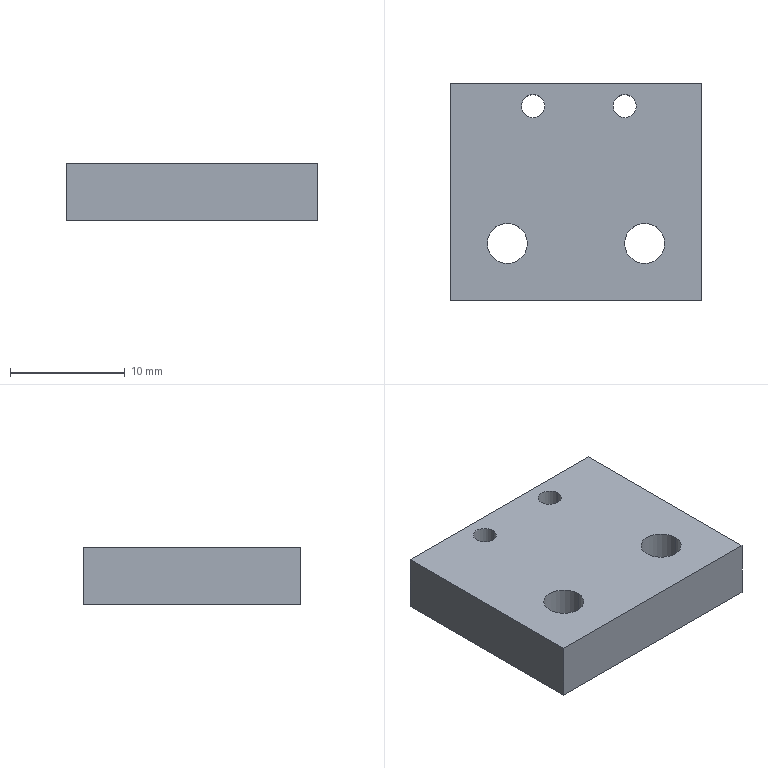Part | SolidWorks | features BaseBody 1 | 1 solid | 14 faces | box 22 x 19 x 5 mm | volume 1962 mm3 | cylinder 8 | plane 6 | commonest cylinder face diameters 2.013 x4 3.5 x4
STEP:
#1=CARTESIAN_POINT('',(-23.757,7.,0.));
#2=VERTEX_POINT('',#1);
#3=CARTESIAN_POINT('',(-21.744,7.,0.));
#4=VERTEX_POINT('',#3);
#5=CARTESIAN_POINT('',(-22.75,7.,0.));
#6=DIRECTION('',(0.,0.,1.));
#7=DIRECTION('',(1.,0.,0.));
#8=AXIS2_PLACEMENT_3D('',#5,#6,#7);
#9=CIRCLE('',#8,1.007);
#10=EDGE_CURVE('',#2,#4,#9,.T.);
#11=ORIENTED_EDGE('',*,*,#10,.F.);
#12=CARTESIAN_POINT('',(-23.757,7.,5.));
#13=VERTEX_POINT('',#12);
#14=CARTESIAN_POINT('',(-23.757,7.,-24.496));
#15=DIRECTION('',(0.,0.,1.));
#16=VECTOR('',#15,1000.);
#17=LINE('',#14,#16);
#18=EDGE_CURVE('',#2,#13,#17,.T.);
#19=ORIENTED_EDGE('',*,*,#18,.T.);
#20=CARTESIAN_POINT('',(-21.744,7.,5.));
#21=VERTEX_POINT('',#20);
#22=CARTESIAN_POINT('',(-22.75,7.,5.));
#23=DIRECTION('',(0.,0.,-1.));
#24=DIRECTION('',(1.,0.,0.));
#25=AXIS2_PLACEMENT_3D('',#22,#23,#24);
#26=CIRCLE('',#25,1.007);
#27=EDGE_CURVE('',#21,#13,#26,.T.);
#28=ORIENTED_EDGE('',*,*,#27,.F.);
#29=CARTESIAN_POINT('',(-21.744,7.,-24.496));
#30=DIRECTION('',(0.,0.,1.));
#31=VECTOR('',#30,1000.);
#32=LINE('',#29,#31);
#33=EDGE_CURVE('',#4,#21,#32,.T.);
#34=ORIENTED_EDGE('',*,*,#33,.F.);
#35=EDGE_LOOP('',(#11,#19,#28,#34));
#36=FACE_OUTER_BOUND('',#35,.T.);
#37=CARTESIAN_POINT('',(-22.75,7.,-24.496));
#38=DIRECTION('',(0.,0.,1.));
#39=DIRECTION('',(1.,0.,0.));
#40=AXIS2_PLACEMENT_3D('',#37,#38,#39);
#41=CYLINDRICAL_SURFACE('',#40,1.007);
#42=ADVANCED_FACE('',(#36),#41,.F.);
#43=CARTESIAN_POINT('',(-15.757,7.,0.));
#44=VERTEX_POINT('',#43);
#45=CARTESIAN_POINT('',(-13.744,7.,0.));
#46=VERTEX_POINT('',#45);
#47=CARTESIAN_POINT('',(-14.75,7.,0.));
#48=DIRECTION('',(0.,0.,1.));
#49=DIRECTION('',(1.,0.,0.));
#50=AXIS2_PLACEMENT_3D('',#47,#48,#49);
#51=CIRCLE('',#50,1.007);
#52=EDGE_CURVE('',#44,#46,#51,.T.);
#53=ORIENTED_EDGE('',*,*,#52,.F.);
#54=CARTESIAN_POINT('',(-15.757,7.,5.));
#55=VERTEX_POINT('',#54);
#56=CARTESIAN_POINT('',(-15.757,7.,-24.496));
#57=DIRECTION('',(0.,0.,1.));
#58=VECTOR('',#57,1000.);
#59=LINE('',#56,#58);
#60=EDGE_CURVE('',#44,#55,#59,.T.);
#61=ORIENTED_EDGE('',*,*,#60,.T.);
#62=CARTESIAN_POINT('',(-13.744,7.,5.));
#63=VERTEX_POINT('',#62);
#64=CARTESIAN_POINT('',(-14.75,7.,5.));
#65=DIRECTION('',(0.,0.,-1.));
#66=DIRECTION('',(1.,0.,0.));
#67=AXIS2_PLACEMENT_3D('',#64,#65,#66);
#68=CIRCLE('',#67,1.007);
#69=EDGE_CURVE('',#63,#55,#68,.T.);
#70=ORIENTED_EDGE('',*,*,#69,.F.);
#71=CARTESIAN_POINT('',(-13.744,7.,-24.496));
#72=DIRECTION('',(0.,0.,1.));
#73=VECTOR('',#72,1000.);
#74=LINE('',#71,#73);
#75=EDGE_CURVE('',#46,#63,#74,.T.);
#76=ORIENTED_EDGE('',*,*,#75,.F.);
#77=EDGE_LOOP('',(#53,#61,#70,#76));
#78=FACE_OUTER_BOUND('',#77,.T.);
#79=CARTESIAN_POINT('',(-14.75,7.,-24.496));
#80=DIRECTION('',(0.,0.,1.));
#81=DIRECTION('',(1.,0.,0.));
#82=AXIS2_PLACEMENT_3D('',#79,#80,#81);
#83=CYLINDRICAL_SURFACE('',#82,1.007);
#84=ADVANCED_FACE('',(#78),#83,.F.);
#85=CARTESIAN_POINT('',(-26.75,-5.,0.));
#86=VERTEX_POINT('',#85);
#87=CARTESIAN_POINT('',(-23.25,-5.,0.));
#88=VERTEX_POINT('',#87);
#89=CARTESIAN_POINT('',(-25.,-5.,0.));
#90=DIRECTION('',(0.,0.,1.));
#91=DIRECTION('',(1.,0.,0.));
#92=AXIS2_PLACEMENT_3D('',#89,#90,#91);
#93=CIRCLE('',#92,1.75);
#94=EDGE_CURVE('',#86,#88,#93,.T.);
#95=ORIENTED_EDGE('',*,*,#94,.F.);
#96=CARTESIAN_POINT('',(-26.75,-5.,5.));
#97=VERTEX_POINT('',#96);
#98=CARTESIAN_POINT('',(-26.75,-5.,-24.496));
#99=DIRECTION('',(0.,0.,1.));
#100=VECTOR('',#99,1000.);
#101=LINE('',#98,#100);
#102=EDGE_CURVE('',#86,#97,#101,.T.);
#103=ORIENTED_EDGE('',*,*,#102,.T.);
#104=CARTESIAN_POINT('',(-23.25,-5.,5.));
#105=VERTEX_POINT('',#104);
#106=CARTESIAN_POINT('',(-25.,-5.,5.));
#107=DIRECTION('',(0.,0.,-1.));
#108=DIRECTION('',(1.,0.,0.));
#109=AXIS2_PLACEMENT_3D('',#106,#107,#108);
#110=CIRCLE('',#109,1.75);
#111=EDGE_CURVE('',#105,#97,#110,.T.);
#112=ORIENTED_EDGE('',*,*,#111,.F.);
#113=CARTESIAN_POINT('',(-23.25,-5.,-24.496));
#114=DIRECTION('',(0.,0.,1.));
#115=VECTOR('',#114,1000.);
#116=LINE('',#113,#115);
#117=EDGE_CURVE('',#88,#105,#116,.T.);
#118=ORIENTED_EDGE('',*,*,#117,.F.);
#119=EDGE_LOOP('',(#95,#103,#112,#118));
#120=FACE_OUTER_BOUND('',#119,.T.);
#121=CARTESIAN_POINT('',(-25.,-5.,-24.496));
#122=DIRECTION('',(0.,0.,1.));
#123=DIRECTION('',(1.,0.,0.));
#124=AXIS2_PLACEMENT_3D('',#121,#122,#123);
#125=CYLINDRICAL_SURFACE('',#124,1.75);
#126=ADVANCED_FACE('',(#120),#125,.F.);
#127=CARTESIAN_POINT('',(-14.75,-5.,0.));
#128=VERTEX_POINT('',#127);
#129=CARTESIAN_POINT('',(-11.25,-5.,0.));
#130=VERTEX_POINT('',#129);
#131=CARTESIAN_POINT('',(-13.,-5.,0.));
#132=DIRECTION('',(0.,0.,1.));
#133=DIRECTION('',(1.,0.,0.));
#134=AXIS2_PLACEMENT_3D('',#131,#132,#133);
#135=CIRCLE('',#134,1.75);
#136=EDGE_CURVE('',#128,#130,#135,.T.);
#137=ORIENTED_EDGE('',*,*,#136,.F.);
#138=CARTESIAN_POINT('',(-14.75,-5.,5.));
#139=VERTEX_POINT('',#138);
#140=CARTESIAN_POINT('',(-14.75,-5.,-24.496));
#141=DIRECTION('',(0.,0.,1.));
#142=VECTOR('',#141,1000.);
#143=LINE('',#140,#142);
#144=EDGE_CURVE('',#128,#139,#143,.T.);
#145=ORIENTED_EDGE('',*,*,#144,.T.);
#146=CARTESIAN_POINT('',(-11.25,-5.,5.));
#147=VERTEX_POINT('',#146);
#148=CARTESIAN_POINT('',(-13.,-5.,5.));
#149=DIRECTION('',(0.,0.,-1.));
#150=DIRECTION('',(1.,0.,0.));
#151=AXIS2_PLACEMENT_3D('',#148,#149,#150);
#152=CIRCLE('',#151,1.75);
#153=EDGE_CURVE('',#147,#139,#152,.T.);
#154=ORIENTED_EDGE('',*,*,#153,.F.);
#155=CARTESIAN_POINT('',(-11.25,-5.,-24.496));
#156=DIRECTION('',(0.,0.,1.));
#157=VECTOR('',#156,1000.);
#158=LINE('',#155,#157);
#159=EDGE_CURVE('',#130,#147,#158,.T.);
#160=ORIENTED_EDGE('',*,*,#159,.F.);
#161=EDGE_LOOP('',(#137,#145,#154,#160));
#162=FACE_OUTER_BOUND('',#161,.T.);
#163=CARTESIAN_POINT('',(-13.,-5.,-24.496));
#164=DIRECTION('',(0.,0.,1.));
#165=DIRECTION('',(1.,0.,0.));
#166=AXIS2_PLACEMENT_3D('',#163,#164,#165);
#167=CYLINDRICAL_SURFACE('',#166,1.75);
#168=ADVANCED_FACE('',(#162),#167,.F.);
#169=ORIENTED_EDGE('',*,*,#27,.T.);
#170=CARTESIAN_POINT('',(-22.75,7.,5.));
#171=DIRECTION('',(0.,0.,-1.));
#172=DIRECTION('',(1.,0.,0.));
#173=AXIS2_PLACEMENT_3D('',#170,#171,#172);
#174=CIRCLE('',#173,1.007);
#175=EDGE_CURVE('',#13,#21,#174,.T.);
#176=ORIENTED_EDGE('',*,*,#175,.T.);
#177=EDGE_LOOP('',(#169,#176));
#178=FACE_BOUND('',#177,.T.);
#179=ORIENTED_EDGE('',*,*,#69,.T.);
#180=CARTESIAN_POINT('',(-14.75,7.,5.));
#181=DIRECTION('',(0.,0.,-1.));
#182=DIRECTION('',(1.,0.,0.));
#183=AXIS2_PLACEMENT_3D('',#180,#181,#182);
#184=CIRCLE('',#183,1.007);
#185=EDGE_CURVE('',#55,#63,#184,.T.);
#186=ORIENTED_EDGE('',*,*,#185,.T.);
#187=EDGE_LOOP('',(#179,#186));
#188=FACE_BOUND('',#187,.T.);
#189=ORIENTED_EDGE('',*,*,#111,.T.);
#190=CARTESIAN_POINT('',(-25.,-5.,5.));
#191=DIRECTION('',(0.,0.,-1.));
#192=DIRECTION('',(1.,0.,0.));
#193=AXIS2_PLACEMENT_3D('',#190,#191,#192);
#194=CIRCLE('',#193,1.75);
#195=EDGE_CURVE('',#97,#105,#194,.T.);
#196=ORIENTED_EDGE('',*,*,#195,.T.);
#197=EDGE_LOOP('',(#189,#196));
#198=FACE_BOUND('',#197,.T.);
#199=ORIENTED_EDGE('',*,*,#153,.T.);
#200=CARTESIAN_POINT('',(-13.,-5.,5.));
#201=DIRECTION('',(0.,0.,-1.));
#202=DIRECTION('',(1.,0.,0.));
#203=AXIS2_PLACEMENT_3D('',#200,#201,#202);
#204=CIRCLE('',#203,1.75);
#205=EDGE_CURVE('',#139,#147,#204,.T.);
#206=ORIENTED_EDGE('',*,*,#205,.T.);
#207=EDGE_LOOP('',(#199,#206));
#208=FACE_BOUND('',#207,.T.);
#209=CARTESIAN_POINT('',(-8.,-10.,5.));
#210=VERTEX_POINT('',#209);
#211=CARTESIAN_POINT('',(-8.,9.,5.));
#212=VERTEX_POINT('',#211);
#213=CARTESIAN_POINT('',(-8.,-0.5,5.));
#214=DIRECTION('',(0.,1.,0.));
#215=VECTOR('',#214,1000.);
#216=LINE('',#213,#215);
#217=EDGE_CURVE('',#210,#212,#216,.T.);
#218=ORIENTED_EDGE('',*,*,#217,.T.);
#219=CARTESIAN_POINT('',(-30.,9.,5.));
#220=VERTEX_POINT('',#219);
#221=CARTESIAN_POINT('',(-19.,9.,5.));
#222=DIRECTION('',(-1.,0.,0.));
#223=VECTOR('',#222,1000.);
#224=LINE('',#221,#223);
#225=EDGE_CURVE('',#212,#220,#224,.T.);
#226=ORIENTED_EDGE('',*,*,#225,.T.);
#227=CARTESIAN_POINT('',(-30.,-10.,5.));
#228=VERTEX_POINT('',#227);
#229=CARTESIAN_POINT('',(-30.,-0.5,5.));
#230=DIRECTION('',(0.,-1.,0.));
#231=VECTOR('',#230,1000.);
#232=LINE('',#229,#231);
#233=EDGE_CURVE('',#220,#228,#232,.T.);
#234=ORIENTED_EDGE('',*,*,#233,.T.);
#235=CARTESIAN_POINT('',(-19.,-10.,5.));
#236=DIRECTION('',(1.,0.,0.));
#237=VECTOR('',#236,1000.);
#238=LINE('',#235,#237);
#239=EDGE_CURVE('',#228,#210,#238,.T.);
#240=ORIENTED_EDGE('',*,*,#239,.T.);
#241=EDGE_LOOP('',(#218,#226,#234,#240));
#242=FACE_OUTER_BOUND('',#241,.T.);
#243=CARTESIAN_POINT('',(-19.,-0.5,5.));
#244=DIRECTION('',(0.,0.,1.));
#245=DIRECTION('',(1.,0.,0.));
#246=AXIS2_PLACEMENT_3D('',#243,#244,#245);
#247=PLANE('',#246);
#248=ADVANCED_FACE('',(#178,#188,#198,#208,#242),#247,.T.);
#249=ORIENTED_EDGE('',*,*,#18,.F.);
#250=CARTESIAN_POINT('',(-22.75,7.,0.));
#251=DIRECTION('',(0.,0.,1.));
#252=DIRECTION('',(1.,0.,0.));
#253=AXIS2_PLACEMENT_3D('',#250,#251,#252);
#254=CIRCLE('',#253,1.007);
#255=EDGE_CURVE('',#4,#2,#254,.T.);
#256=ORIENTED_EDGE('',*,*,#255,.F.);
#257=ORIENTED_EDGE('',*,*,#33,.T.);
#258=ORIENTED_EDGE('',*,*,#175,.F.);
#259=EDGE_LOOP('',(#249,#256,#257,#258));
#260=FACE_OUTER_BOUND('',#259,.T.);
#261=CARTESIAN_POINT('',(-22.75,7.,-24.496));
#262=DIRECTION('',(0.,0.,1.));
#263=DIRECTION('',(1.,0.,0.));
#264=AXIS2_PLACEMENT_3D('',#261,#262,#263);
#265=CYLINDRICAL_SURFACE('',#264,1.007);
#266=ADVANCED_FACE('',(#260),#265,.F.);
#267=ORIENTED_EDGE('',*,*,#60,.F.);
#268=CARTESIAN_POINT('',(-14.75,7.,0.));
#269=DIRECTION('',(0.,0.,1.));
#270=DIRECTION('',(1.,0.,0.));
#271=AXIS2_PLACEMENT_3D('',#268,#269,#270);
#272=CIRCLE('',#271,1.007);
#273=EDGE_CURVE('',#46,#44,#272,.T.);
#274=ORIENTED_EDGE('',*,*,#273,.F.);
#275=ORIENTED_EDGE('',*,*,#75,.T.);
#276=ORIENTED_EDGE('',*,*,#185,.F.);
#277=EDGE_LOOP('',(#267,#274,#275,#276));
#278=FACE_OUTER_BOUND('',#277,.T.);
#279=CARTESIAN_POINT('',(-14.75,7.,-24.496));
#280=DIRECTION('',(0.,0.,1.));
#281=DIRECTION('',(1.,0.,0.));
#282=AXIS2_PLACEMENT_3D('',#279,#280,#281);
#283=CYLINDRICAL_SURFACE('',#282,1.007);
#284=ADVANCED_FACE('',(#278),#283,.F.);
#285=ORIENTED_EDGE('',*,*,#102,.F.);
#286=CARTESIAN_POINT('',(-25.,-5.,0.));
#287=DIRECTION('',(0.,0.,1.));
#288=DIRECTION('',(1.,0.,0.));
#289=AXIS2_PLACEMENT_3D('',#286,#287,#288);
#290=CIRCLE('',#289,1.75);
#291=EDGE_CURVE('',#88,#86,#290,.T.);
#292=ORIENTED_EDGE('',*,*,#291,.F.);
#293=ORIENTED_EDGE('',*,*,#117,.T.);
#294=ORIENTED_EDGE('',*,*,#195,.F.);
#295=EDGE_LOOP('',(#285,#292,#293,#294));
#296=FACE_OUTER_BOUND('',#295,.T.);
#297=CARTESIAN_POINT('',(-25.,-5.,-24.496));
#298=DIRECTION('',(0.,0.,1.));
#299=DIRECTION('',(1.,0.,0.));
#300=AXIS2_PLACEMENT_3D('',#297,#298,#299);
#301=CYLINDRICAL_SURFACE('',#300,1.75);
#302=ADVANCED_FACE('',(#296),#301,.F.);
#303=ORIENTED_EDGE('',*,*,#144,.F.);
#304=CARTESIAN_POINT('',(-13.,-5.,0.));
#305=DIRECTION('',(0.,0.,1.));
#306=DIRECTION('',(1.,0.,0.));
#307=AXIS2_PLACEMENT_3D('',#304,#305,#306);
#308=CIRCLE('',#307,1.75);
#309=EDGE_CURVE('',#130,#128,#308,.T.);
#310=ORIENTED_EDGE('',*,*,#309,.F.);
#311=ORIENTED_EDGE('',*,*,#159,.T.);
#312=ORIENTED_EDGE('',*,*,#205,.F.);
#313=EDGE_LOOP('',(#303,#310,#311,#312));
#314=FACE_OUTER_BOUND('',#313,.T.);
#315=CARTESIAN_POINT('',(-13.,-5.,-24.496));
#316=DIRECTION('',(0.,0.,1.));
#317=DIRECTION('',(1.,0.,0.));
#318=AXIS2_PLACEMENT_3D('',#315,#316,#317);
#319=CYLINDRICAL_SURFACE('',#318,1.75);
#320=ADVANCED_FACE('',(#314),#319,.F.);
#321=CARTESIAN_POINT('',(-8.,9.,0.));
#322=VERTEX_POINT('',#321);
#323=CARTESIAN_POINT('',(-30.,9.,0.));
#324=VERTEX_POINT('',#323);
#325=CARTESIAN_POINT('',(-30.,9.,0.));
#326=DIRECTION('',(-1.,0.,0.));
#327=VECTOR('',#326,1000.);
#328=LINE('',#325,#327);
#329=EDGE_CURVE('',#322,#324,#328,.T.);
#330=ORIENTED_EDGE('',*,*,#329,.T.);
#331=CARTESIAN_POINT('',(-30.,9.,0.));
#332=DIRECTION('',(0.,0.,1.));
#333=VECTOR('',#332,1000.);
#334=LINE('',#331,#333);
#335=EDGE_CURVE('',#324,#220,#334,.T.);
#336=ORIENTED_EDGE('',*,*,#335,.T.);
#337=ORIENTED_EDGE('',*,*,#225,.F.);
#338=CARTESIAN_POINT('',(-8.,9.,0.));
#339=DIRECTION('',(0.,0.,-1.));
#340=VECTOR('',#339,1000.);
#341=LINE('',#338,#340);
#342=EDGE_CURVE('',#212,#322,#341,.T.);
#343=ORIENTED_EDGE('',*,*,#342,.T.);
#344=EDGE_LOOP('',(#330,#336,#337,#343));
#345=FACE_OUTER_BOUND('',#344,.T.);
#346=CARTESIAN_POINT('',(-30.,9.,0.));
#347=DIRECTION('',(0.,1.,0.));
#348=DIRECTION('',(0.,0.,1.));
#349=AXIS2_PLACEMENT_3D('',#346,#347,#348);
#350=PLANE('',#349);
#351=ADVANCED_FACE('',(#345),#350,.T.);
#352=CARTESIAN_POINT('',(-8.,-10.,0.));
#353=VERTEX_POINT('',#352);
#354=CARTESIAN_POINT('',(-8.,9.,0.));
#355=DIRECTION('',(0.,1.,0.));
#356=VECTOR('',#355,1000.);
#357=LINE('',#354,#356);
#358=EDGE_CURVE('',#353,#322,#357,.T.);
#359=ORIENTED_EDGE('',*,*,#358,.T.);
#360=ORIENTED_EDGE('',*,*,#342,.F.);
#361=ORIENTED_EDGE('',*,*,#217,.F.);
#362=CARTESIAN_POINT('',(-8.,-10.,0.));
#363=DIRECTION('',(0.,0.,-1.));
#364=VECTOR('',#363,1000.);
#365=LINE('',#362,#364);
#366=EDGE_CURVE('',#210,#353,#365,.T.);
#367=ORIENTED_EDGE('',*,*,#366,.T.);
#368=EDGE_LOOP('',(#359,#360,#361,#367));
#369=FACE_OUTER_BOUND('',#368,.T.);
#370=CARTESIAN_POINT('',(-8.,9.,0.));
#371=DIRECTION('',(1.,0.,0.));
#372=DIRECTION('',(0.,0.,-1.));
#373=AXIS2_PLACEMENT_3D('',#370,#371,#372);
#374=PLANE('',#373);
#375=ADVANCED_FACE('',(#369),#374,.T.);
#376=CARTESIAN_POINT('',(-30.,-10.,0.));
#377=VERTEX_POINT('',#376);
#378=CARTESIAN_POINT('',(-8.,-10.,0.));
#379=DIRECTION('',(1.,0.,0.));
#380=VECTOR('',#379,1000.);
#381=LINE('',#378,#380);
#382=EDGE_CURVE('',#377,#353,#381,.T.);
#383=ORIENTED_EDGE('',*,*,#382,.T.);
#384=ORIENTED_EDGE('',*,*,#366,.F.);
#385=ORIENTED_EDGE('',*,*,#239,.F.);
#386=CARTESIAN_POINT('',(-30.,-10.,0.));
#387=DIRECTION('',(0.,0.,-1.));
#388=VECTOR('',#387,1000.);
#389=LINE('',#386,#388);
#390=EDGE_CURVE('',#228,#377,#389,.T.);
#391=ORIENTED_EDGE('',*,*,#390,.T.);
#392=EDGE_LOOP('',(#383,#384,#385,#391));
#393=FACE_OUTER_BOUND('',#392,.T.);
#394=CARTESIAN_POINT('',(-8.,-10.,0.));
#395=DIRECTION('',(0.,-1.,0.));
#396=DIRECTION('',(0.,0.,-1.));
#397=AXIS2_PLACEMENT_3D('',#394,#395,#396);
#398=PLANE('',#397);
#399=ADVANCED_FACE('',(#393),#398,.T.);
#400=CARTESIAN_POINT('',(-30.,-10.,0.));
#401=DIRECTION('',(0.,-1.,0.));
#402=VECTOR('',#401,1000.);
#403=LINE('',#400,#402);
#404=EDGE_CURVE('',#324,#377,#403,.T.);
#405=ORIENTED_EDGE('',*,*,#404,.T.);
#406=ORIENTED_EDGE('',*,*,#390,.F.);
#407=ORIENTED_EDGE('',*,*,#233,.F.);
#408=ORIENTED_EDGE('',*,*,#335,.F.);
#409=EDGE_LOOP('',(#405,#406,#407,#408));
#410=FACE_OUTER_BOUND('',#409,.T.);
#411=CARTESIAN_POINT('',(-30.,-10.,0.));
#412=DIRECTION('',(-1.,0.,0.));
#413=DIRECTION('',(0.,0.,1.));
#414=AXIS2_PLACEMENT_3D('',#411,#412,#413);
#415=PLANE('',#414);
#416=ADVANCED_FACE('',(#410),#415,.T.);
#417=ORIENTED_EDGE('',*,*,#255,.T.);
#418=ORIENTED_EDGE('',*,*,#10,.T.);
#419=EDGE_LOOP('',(#417,#418));
#420=FACE_BOUND('',#419,.T.);
#421=ORIENTED_EDGE('',*,*,#273,.T.);
#422=ORIENTED_EDGE('',*,*,#52,.T.);
#423=EDGE_LOOP('',(#421,#422));
#424=FACE_BOUND('',#423,.T.);
#425=ORIENTED_EDGE('',*,*,#291,.T.);
#426=ORIENTED_EDGE('',*,*,#94,.T.);
#427=EDGE_LOOP('',(#425,#426));
#428=FACE_BOUND('',#427,.T.);
#429=ORIENTED_EDGE('',*,*,#309,.T.);
#430=ORIENTED_EDGE('',*,*,#136,.T.);
#431=EDGE_LOOP('',(#429,#430));
#432=FACE_BOUND('',#431,.T.);
#433=ORIENTED_EDGE('',*,*,#404,.F.);
#434=ORIENTED_EDGE('',*,*,#329,.F.);
#435=ORIENTED_EDGE('',*,*,#358,.F.);
#436=ORIENTED_EDGE('',*,*,#382,.F.);
#437=EDGE_LOOP('',(#433,#434,#435,#436));
#438=FACE_OUTER_BOUND('',#437,.T.);
#439=CARTESIAN_POINT('',(-19.,-0.5,0.));
#440=DIRECTION('',(0.,0.,1.));
#441=DIRECTION('',(1.,0.,0.));
#442=AXIS2_PLACEMENT_3D('',#439,#440,#441);
#443=PLANE('',#442);
#444=ADVANCED_FACE('',(#420,#424,#428,#432,#438),#443,.F.);
#445=CLOSED_SHELL('',(#42,#84,#126,#168,#248,#266,#284,#302,#320,#351,#375,#399,#416,#444));
#446=MANIFOLD_SOLID_BREP('',#445);
#447=CARTESIAN_POINT('',(0.,0.,0.));
#448=DIRECTION('',(0.,0.,1.));
#449=DIRECTION('',(1.,0.,0.));
#450=AXIS2_PLACEMENT_3D('',#447,#448,#449);
#451=(LENGTH_UNIT()NAMED_UNIT(*)SI_UNIT(.MILLI.,.METRE.));
#452=UNCERTAINTY_MEASURE_WITH_UNIT(LENGTH_MEASURE(0.00001),#451,'','');
#453=(NAMED_UNIT(*)PLANE_ANGLE_UNIT()SI_UNIT($,.RADIAN.));
#454=(NAMED_UNIT(*)SI_UNIT($,.STERADIAN.)SOLID_ANGLE_UNIT());
#455=(GEOMETRIC_REPRESENTATION_CONTEXT(3)GLOBAL_UNCERTAINTY_ASSIGNED_CONTEXT((#452))GLOBAL_UNIT_ASSIGNED_CONTEXT((#451,#453,#454))REPRESENTATION_CONTEXT('',''));
#456=ADVANCED_BREP_SHAPE_REPRESENTATION('',(#446,#450),#455);